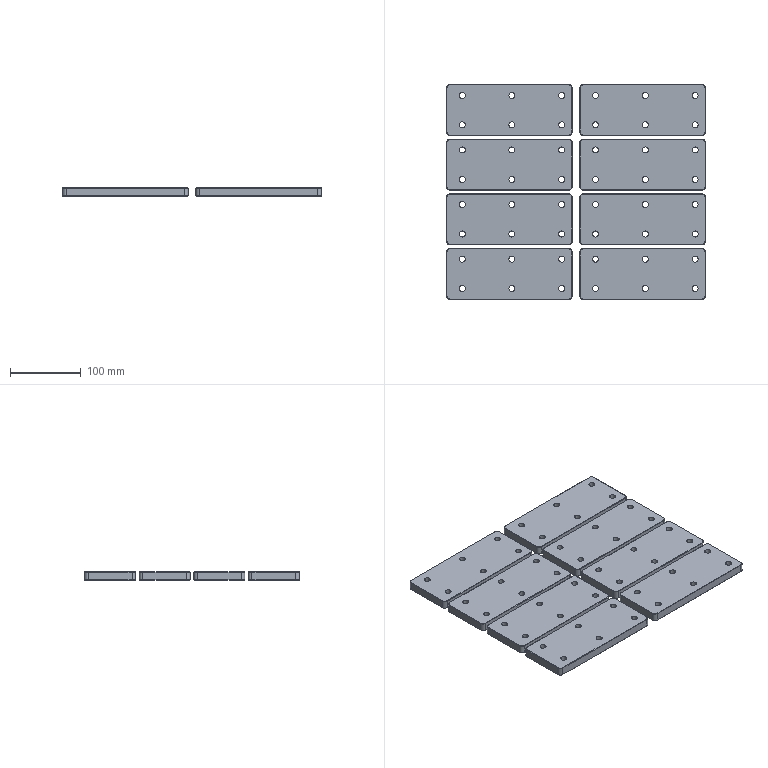CAM job | NX | 3-axis milling | part box 365 x 303 x 12 mm | stock box 369 x 307 x 12 mm
Operations:
program,operation,operation_type,tool,method,geometry_group,spindle_rpm,surface_speed,feed_per_tooth,feed_cut,feed_plunge,cut_length_mm,path_length_mm,cut_time_min,machine_time_min
1吸,ZLEVEL_PROFILE_1_COPY_1_COPY,ZLevelMilling,D4A45,METHOD,A,9500.0,179.0,0.0526,1000.0,100.0,5180.45,15472.264,5.18,6.21
1吸,HOLE_MILLING,CylinderMilling,D6,METHOD,A,9500.0,179.0,0.0658,1250.0,100.0,9896.018,15350.167,7.917,8.462
1吸,ZLEVEL_PROFILE_COPY_COPY_1_COPY,ZLevelMilling,D4,METHOD,A,9500.0,119.0,0.1158,2200.0,1000.0,120954.544,122919.267,55.137,55.334